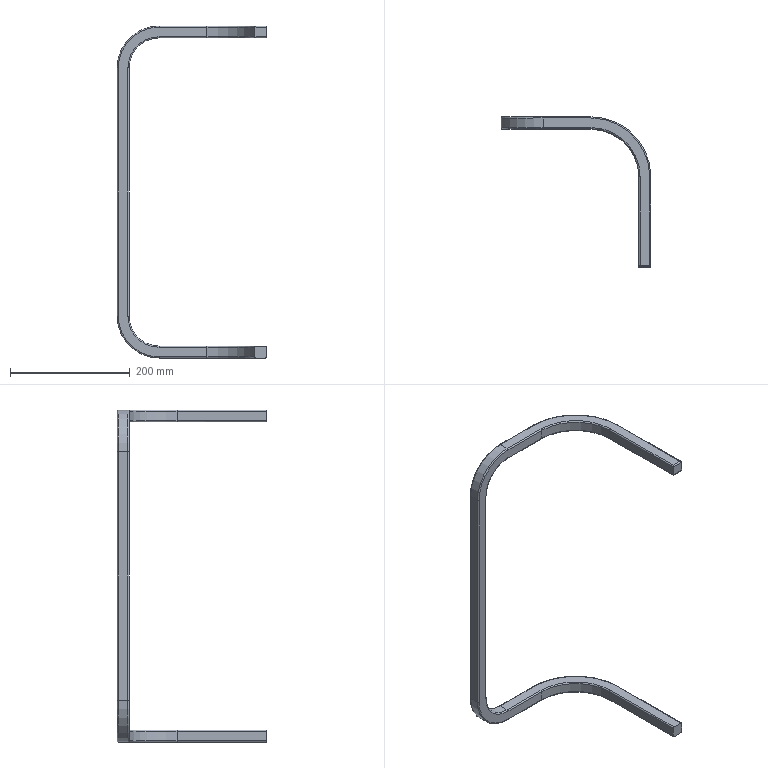Part | SolidWorks | features Fillet 3, Extrusion 1, ICE 1 | 1 solid | 60 faces | box 250 x 250 x 554 mm | volume 533445 mm3 | cylinder 30 | torus 16 | plane 14 | commonest cylinder face diameters 4 x22 100 x2 140 x2 160 x2 200 x2